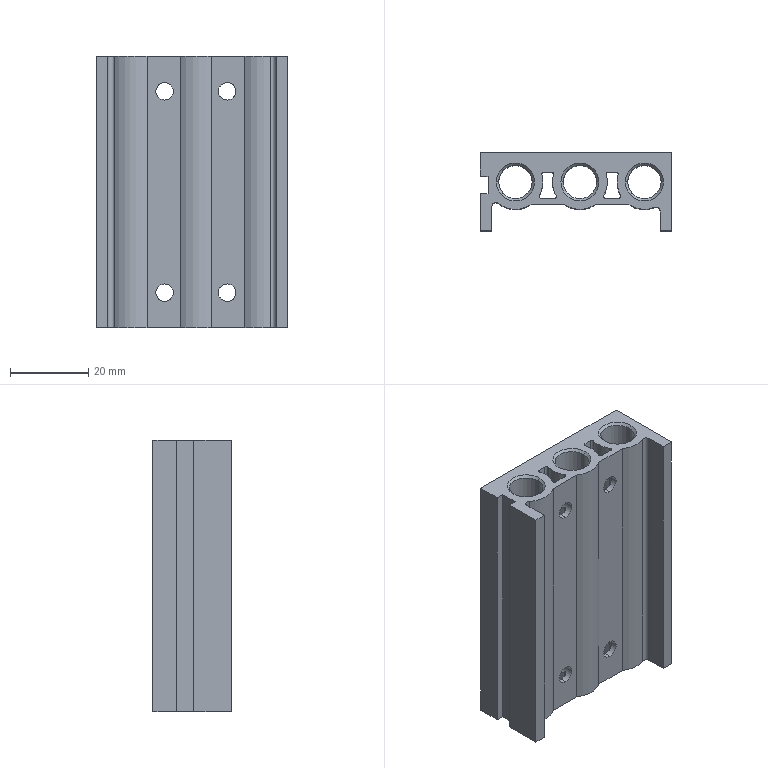Part | STEP file | Solenoid Valve Manifold SS5Y3-20-04_Default | 1 solid | 132 faces | box 49 x 20 x 69.5 mm | volume 33276 mm3 | cylinder 85 | plane 35 | cone 12 | commonest cylinder face diameters 1 x32 14 x17 1.25 x16 4.5 x12 8.57 x6 2 x2